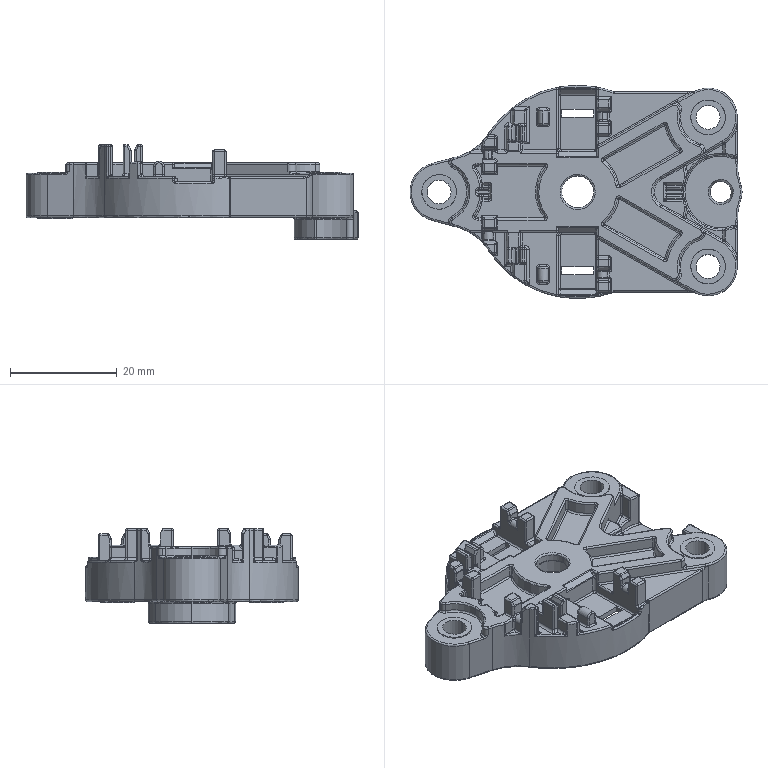Part | SolidWorks | features BaseBody 1 | 1 solid | 1571 faces | box 62.36 x 40 x 17.8 mm | volume 10187 mm3 | cylinder 657 | spline 519 | plane 236 | torus 157 | cone 2 | commonest cylinder face diameters 0.6 x502 2 x27 1 x23 0.2 x12 6.5 x12 11 x11